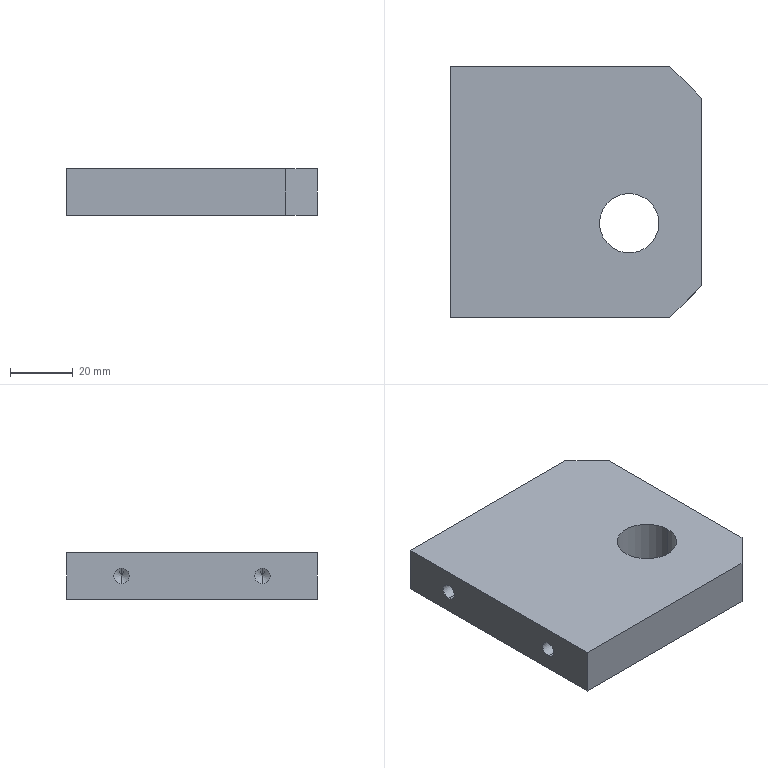Part | STEP file | Lead screw rear fixing plate | 1 solid | 18 faces | box 80 x 80 x 15 mm | volume 89638 mm3 | plane 8 | cylinder 6 | cone 4 | commonest cylinder face diameters 5 x4 19 x2
STEP:
#1=CARTESIAN_POINT('',(0.,0.,0.));
#2=DIRECTION('',(0.,0.,1.));
#3=DIRECTION('',(1.,0.,0.));
#4=AXIS2_PLACEMENT_3D('',#1,#2,#3);
#5=CARTESIAN_POINT('',(-106.907,13.444,5.));
#6=VERTEX_POINT('',#5);
#7=CARTESIAN_POINT('',(-106.907,13.444,10.));
#8=VERTEX_POINT('',#7);
#9=CARTESIAN_POINT('',(-106.907,13.444,7.5));
#10=DIRECTION('',(-1.,0.,0.));
#11=DIRECTION('',(0.,0.,1.));
#12=AXIS2_PLACEMENT_3D('',#9,#10,#11);
#13=CIRCLE('',#12,2.5);
#14=CARTESIAN_POINT('',(-106.907,13.444,7.5));
#15=DIRECTION('',(-1.,0.,0.));
#16=DIRECTION('',(0.,0.,1.));
#17=AXIS2_PLACEMENT_3D('',#14,#15,#16);
#18=CONICAL_SURFACE('',#17,2.5,1.03);
#19=CARTESIAN_POINT('',(0.,0.));
#20=DIRECTION('',(1.,0.));
#21=VECTOR('',#20,1.);
#22=LINE('',#19,#21);
#23=(GEOMETRIC_REPRESENTATION_CONTEXT(2)PARAMETRIC_REPRESENTATION_CONTEXT()REPRESENTATION_CONTEXT('',''));
#24=DEFINITIONAL_REPRESENTATION('',(#22),#23);
#25=PCURVE('',#18,#24);
#26=CARTESIAN_POINT('',(-106.907,13.444,7.5));
#27=DIRECTION('',(-1.,0.,0.));
#28=DIRECTION('',(0.,0.,1.));
#29=AXIS2_PLACEMENT_3D('',#26,#27,#28);
#30=CYLINDRICAL_SURFACE('',#29,2.5);
#31=CARTESIAN_POINT('',(0.,0.));
#32=DIRECTION('',(1.,0.));
#33=VECTOR('',#32,1.);
#34=LINE('',#31,#33);
#35=(GEOMETRIC_REPRESENTATION_CONTEXT(2)PARAMETRIC_REPRESENTATION_CONTEXT()REPRESENTATION_CONTEXT('',''));
#36=DEFINITIONAL_REPRESENTATION('',(#34),#35);
#37=PCURVE('',#30,#36);
#38=SURFACE_CURVE('',#13,(#25,#37),.PCURVE_S1.);
#39=EDGE_CURVE('',#6,#8,#38,.T.);
#40=ORIENTED_EDGE('',*,*,#39,.F.);
#41=CARTESIAN_POINT('',(-105.405,13.444,7.5));
#42=VERTEX_POINT('',#41);
#43=CARTESIAN_POINT('',(-106.907,13.444,5.));
#44=DIRECTION('',(-0.515,0.,-0.8572));
#45=VECTOR('',#44,1.);
#46=LINE('',#43,#45);
#47=CARTESIAN_POINT('',(3.142,0.));
#48=DIRECTION('',(0.,1.));
#49=VECTOR('',#48,1.);
#50=LINE('',#47,#49);
#51=(GEOMETRIC_REPRESENTATION_CONTEXT(2)PARAMETRIC_REPRESENTATION_CONTEXT()REPRESENTATION_CONTEXT('',''));
#52=DEFINITIONAL_REPRESENTATION('',(#50),#51);
#53=PCURVE('',#18,#52);
#54=CARTESIAN_POINT('',(-106.907,13.444,7.5));
#55=DIRECTION('',(-1.,0.,0.));
#56=DIRECTION('',(0.,0.,1.));
#57=AXIS2_PLACEMENT_3D('',#54,#55,#56);
#58=CONICAL_SURFACE('',#57,2.5,1.03);
#59=CARTESIAN_POINT('',(3.142,0.));
#60=DIRECTION('',(0.,1.));
#61=VECTOR('',#60,1.);
#62=LINE('',#59,#61);
#63=(GEOMETRIC_REPRESENTATION_CONTEXT(2)PARAMETRIC_REPRESENTATION_CONTEXT()REPRESENTATION_CONTEXT('',''));
#64=DEFINITIONAL_REPRESENTATION('',(#62),#63);
#65=PCURVE('',#58,#64);
#66=SURFACE_CURVE('',#46,(#53,#65),.PCURVE_S1.);
#67=EDGE_CURVE('',#42,#6,#66,.T.);
#68=ORIENTED_EDGE('',*,*,#67,.F.);
#69=CARTESIAN_POINT('',(-106.907,13.444,10.));
#70=DIRECTION('',(-0.515,0.,0.8572));
#71=VECTOR('',#70,1.);
#72=LINE('',#69,#71);
#73=CARTESIAN_POINT('',(6.283,0.));
#74=DIRECTION('',(0.,1.));
#75=VECTOR('',#74,1.);
#76=LINE('',#73,#75);
#77=(GEOMETRIC_REPRESENTATION_CONTEXT(2)PARAMETRIC_REPRESENTATION_CONTEXT()REPRESENTATION_CONTEXT('',''));
#78=DEFINITIONAL_REPRESENTATION('',(#76),#77);
#79=PCURVE('',#18,#78);
#80=CARTESIAN_POINT('',(0.,0.));
#81=DIRECTION('',(0.,1.));
#82=VECTOR('',#81,1.);
#83=LINE('',#80,#82);
#84=(GEOMETRIC_REPRESENTATION_CONTEXT(2)PARAMETRIC_REPRESENTATION_CONTEXT()REPRESENTATION_CONTEXT('',''));
#85=DEFINITIONAL_REPRESENTATION('',(#83),#84);
#86=PCURVE('',#58,#85);
#87=SURFACE_CURVE('',#72,(#79,#86),.PCURVE_S1.);
#88=EDGE_CURVE('',#42,#8,#87,.T.);
#89=ORIENTED_EDGE('',*,*,#88,.T.);
#90=EDGE_LOOP('',(#40,#68,#89));
#91=FACE_BOUND('',#90,.F.);
#92=ADVANCED_FACE('',(#91),#18,.F.);
#93=CARTESIAN_POINT('',(-106.907,-31.556,5.));
#94=VERTEX_POINT('',#93);
#95=CARTESIAN_POINT('',(-106.907,-31.556,10.));
#96=VERTEX_POINT('',#95);
#97=CARTESIAN_POINT('',(-106.907,-31.556,7.5));
#98=DIRECTION('',(-1.,0.,0.));
#99=DIRECTION('',(0.,0.,1.));
#100=AXIS2_PLACEMENT_3D('',#97,#98,#99);
#101=CIRCLE('',#100,2.5);
#102=CARTESIAN_POINT('',(-106.907,-31.556,7.5));
#103=DIRECTION('',(-1.,0.,0.));
#104=DIRECTION('',(0.,0.,1.));
#105=AXIS2_PLACEMENT_3D('',#102,#103,#104);
#106=CONICAL_SURFACE('',#105,2.5,1.03);
#107=CARTESIAN_POINT('',(0.,0.));
#108=DIRECTION('',(1.,0.));
#109=VECTOR('',#108,1.);
#110=LINE('',#107,#109);
#111=(GEOMETRIC_REPRESENTATION_CONTEXT(2)PARAMETRIC_REPRESENTATION_CONTEXT()REPRESENTATION_CONTEXT('',''));
#112=DEFINITIONAL_REPRESENTATION('',(#110),#111);
#113=PCURVE('',#106,#112);
#114=CARTESIAN_POINT('',(-106.907,-31.556,7.5));
#115=DIRECTION('',(-1.,0.,0.));
#116=DIRECTION('',(0.,0.,1.));
#117=AXIS2_PLACEMENT_3D('',#114,#115,#116);
#118=CYLINDRICAL_SURFACE('',#117,2.5);
#119=CARTESIAN_POINT('',(0.,0.));
#120=DIRECTION('',(1.,0.));
#121=VECTOR('',#120,1.);
#122=LINE('',#119,#121);
#123=(GEOMETRIC_REPRESENTATION_CONTEXT(2)PARAMETRIC_REPRESENTATION_CONTEXT()REPRESENTATION_CONTEXT('',''));
#124=DEFINITIONAL_REPRESENTATION('',(#122),#123);
#125=PCURVE('',#118,#124);
#126=SURFACE_CURVE('',#101,(#113,#125),.PCURVE_S1.);
#127=EDGE_CURVE('',#94,#96,#126,.T.);
#128=ORIENTED_EDGE('',*,*,#127,.F.);
#129=CARTESIAN_POINT('',(-105.405,-31.556,7.5));
#130=VERTEX_POINT('',#129);
#131=CARTESIAN_POINT('',(-106.907,-31.556,5.));
#132=DIRECTION('',(-0.515,0.,-0.8572));
#133=VECTOR('',#132,1.);
#134=LINE('',#131,#133);
#135=CARTESIAN_POINT('',(3.142,0.));
#136=DIRECTION('',(0.,1.));
#137=VECTOR('',#136,1.);
#138=LINE('',#135,#137);
#139=(GEOMETRIC_REPRESENTATION_CONTEXT(2)PARAMETRIC_REPRESENTATION_CONTEXT()REPRESENTATION_CONTEXT('',''));
#140=DEFINITIONAL_REPRESENTATION('',(#138),#139);
#141=PCURVE('',#106,#140);
#142=CARTESIAN_POINT('',(-106.907,-31.556,7.5));
#143=DIRECTION('',(-1.,0.,0.));
#144=DIRECTION('',(0.,0.,1.));
#145=AXIS2_PLACEMENT_3D('',#142,#143,#144);
#146=CONICAL_SURFACE('',#145,2.5,1.03);
#147=CARTESIAN_POINT('',(3.142,0.));
#148=DIRECTION('',(0.,1.));
#149=VECTOR('',#148,1.);
#150=LINE('',#147,#149);
#151=(GEOMETRIC_REPRESENTATION_CONTEXT(2)PARAMETRIC_REPRESENTATION_CONTEXT()REPRESENTATION_CONTEXT('',''));
#152=DEFINITIONAL_REPRESENTATION('',(#150),#151);
#153=PCURVE('',#146,#152);
#154=SURFACE_CURVE('',#134,(#141,#153),.PCURVE_S1.);
#155=EDGE_CURVE('',#130,#94,#154,.T.);
#156=ORIENTED_EDGE('',*,*,#155,.F.);
#157=CARTESIAN_POINT('',(-106.907,-31.556,10.));
#158=DIRECTION('',(-0.515,0.,0.8572));
#159=VECTOR('',#158,1.);
#160=LINE('',#157,#159);
#161=CARTESIAN_POINT('',(6.283,0.));
#162=DIRECTION('',(0.,1.));
#163=VECTOR('',#162,1.);
#164=LINE('',#161,#163);
#165=(GEOMETRIC_REPRESENTATION_CONTEXT(2)PARAMETRIC_REPRESENTATION_CONTEXT()REPRESENTATION_CONTEXT('',''));
#166=DEFINITIONAL_REPRESENTATION('',(#164),#165);
#167=PCURVE('',#106,#166);
#168=CARTESIAN_POINT('',(0.,0.));
#169=DIRECTION('',(0.,1.));
#170=VECTOR('',#169,1.);
#171=LINE('',#168,#170);
#172=(GEOMETRIC_REPRESENTATION_CONTEXT(2)PARAMETRIC_REPRESENTATION_CONTEXT()REPRESENTATION_CONTEXT('',''));
#173=DEFINITIONAL_REPRESENTATION('',(#171),#172);
#174=PCURVE('',#146,#173);
#175=SURFACE_CURVE('',#160,(#167,#174),.PCURVE_S1.);
#176=EDGE_CURVE('',#130,#96,#175,.T.);
#177=ORIENTED_EDGE('',*,*,#176,.T.);
#178=EDGE_LOOP('',(#128,#156,#177));
#179=FACE_BOUND('',#178,.F.);
#180=ADVANCED_FACE('',(#179),#106,.F.);
#181=CARTESIAN_POINT('',(-121.907,-31.556,10.));
#182=VERTEX_POINT('',#181);
#183=CARTESIAN_POINT('',(-106.907,-31.556,10.));
#184=DIRECTION('',(-1.,0.,0.));
#185=VECTOR('',#184,1.);
#186=LINE('',#183,#185);
#187=CARTESIAN_POINT('',(6.283,0.));
#188=DIRECTION('',(0.,1.));
#189=VECTOR('',#188,1.);
#190=LINE('',#187,#189);
#191=(GEOMETRIC_REPRESENTATION_CONTEXT(2)PARAMETRIC_REPRESENTATION_CONTEXT()REPRESENTATION_CONTEXT('',''));
#192=DEFINITIONAL_REPRESENTATION('',(#190),#191);
#193=PCURVE('',#118,#192);
#194=CARTESIAN_POINT('',(-106.907,-31.556,7.5));
#195=DIRECTION('',(-1.,0.,0.));
#196=DIRECTION('',(0.,0.,1.));
#197=AXIS2_PLACEMENT_3D('',#194,#195,#196);
#198=CYLINDRICAL_SURFACE('',#197,2.5);
#199=CARTESIAN_POINT('',(0.,0.));
#200=DIRECTION('',(0.,1.));
#201=VECTOR('',#200,1.);
#202=LINE('',#199,#201);
#203=(GEOMETRIC_REPRESENTATION_CONTEXT(2)PARAMETRIC_REPRESENTATION_CONTEXT()REPRESENTATION_CONTEXT('',''));
#204=DEFINITIONAL_REPRESENTATION('',(#202),#203);
#205=PCURVE('',#198,#204);
#206=SURFACE_CURVE('',#186,(#193,#205),.PCURVE_S1.);
#207=EDGE_CURVE('',#96,#182,#206,.T.);
#208=ORIENTED_EDGE('',*,*,#207,.T.);
#209=CARTESIAN_POINT('',(-121.907,-31.556,5.));
#210=VERTEX_POINT('',#209);
#211=CARTESIAN_POINT('',(-121.907,-31.556,7.5));
#212=DIRECTION('',(-1.,0.,0.));
#213=DIRECTION('',(0.,0.,-1.));
#214=AXIS2_PLACEMENT_3D('',#211,#212,#213);
#215=CIRCLE('',#214,2.5);
#216=CARTESIAN_POINT('',(3.142,15.));
#217=DIRECTION('',(1.,0.));
#218=VECTOR('',#217,1.);
#219=LINE('',#216,#218);
#220=(GEOMETRIC_REPRESENTATION_CONTEXT(2)PARAMETRIC_REPRESENTATION_CONTEXT()REPRESENTATION_CONTEXT('',''));
#221=DEFINITIONAL_REPRESENTATION('',(#219),#220);
#222=PCURVE('',#118,#221);
#223=CARTESIAN_POINT('',(-121.907,-49.056,15.));
#224=DIRECTION('',(1.,0.,0.));
#225=DIRECTION('',(0.,0.,-1.));
#226=AXIS2_PLACEMENT_3D('',#223,#224,#225);
#227=PLANE('',#226);
#228=CARTESIAN_POINT('',(10.,17.5));
#229=CARTESIAN_POINT('',(10.,13.17));
#230=CARTESIAN_POINT('',(6.25,15.335));
#231=CARTESIAN_POINT('',(2.5,17.5));
#232=CARTESIAN_POINT('',(6.25,19.665));
#233=CARTESIAN_POINT('',(10.,21.83));
#234=CARTESIAN_POINT('',(10.,17.5));
#235=(BOUNDED_CURVE()B_SPLINE_CURVE(2,(#228,#229,#230,#231,#232,#233,#234),.UNSPECIFIED.,.T.,.F.)B_SPLINE_CURVE_WITH_KNOTS((1,2,2,2,2,1),(-2.094,0.,2.094,4.189,6.283,8.378),.UNSPECIFIED.)CURVE()GEOMETRIC_REPRESENTATION_ITEM()RATIONAL_B_SPLINE_CURVE((1.,0.5,1.,0.5,1.,0.5,1.))REPRESENTATION_ITEM(''));
#236=(GEOMETRIC_REPRESENTATION_CONTEXT(2)PARAMETRIC_REPRESENTATION_CONTEXT()REPRESENTATION_CONTEXT('',''));
#237=DEFINITIONAL_REPRESENTATION('',(#235),#236);
#238=PCURVE('',#227,#237);
#239=SURFACE_CURVE('',#215,(#222,#238),.PCURVE_S1.);
#240=EDGE_CURVE('',#210,#182,#239,.T.);
#241=ORIENTED_EDGE('',*,*,#240,.F.);
#242=CARTESIAN_POINT('',(-106.907,-31.556,5.));
#243=DIRECTION('',(-1.,0.,0.));
#244=VECTOR('',#243,1.);
#245=LINE('',#242,#244);
#246=CARTESIAN_POINT('',(3.142,0.));
#247=DIRECTION('',(0.,1.));
#248=VECTOR('',#247,1.);
#249=LINE('',#246,#248);
#250=(GEOMETRIC_REPRESENTATION_CONTEXT(2)PARAMETRIC_REPRESENTATION_CONTEXT()REPRESENTATION_CONTEXT('',''));
#251=DEFINITIONAL_REPRESENTATION('',(#249),#250);
#252=PCURVE('',#118,#251);
#253=CARTESIAN_POINT('',(3.142,0.));
#254=DIRECTION('',(0.,1.));
#255=VECTOR('',#254,1.);
#256=LINE('',#253,#255);
#257=(GEOMETRIC_REPRESENTATION_CONTEXT(2)PARAMETRIC_REPRESENTATION_CONTEXT()REPRESENTATION_CONTEXT('',''));
#258=DEFINITIONAL_REPRESENTATION('',(#256),#257);
#259=PCURVE('',#198,#258);
#260=SURFACE_CURVE('',#245,(#252,#259),.PCURVE_S1.);
#261=EDGE_CURVE('',#94,#210,#260,.T.);
#262=ORIENTED_EDGE('',*,*,#261,.F.);
#263=ORIENTED_EDGE('',*,*,#127,.T.);
#264=EDGE_LOOP('',(#208,#241,#262,#263));
#265=FACE_BOUND('',#264,.F.);
#266=ADVANCED_FACE('',(#265),#118,.F.);
#267=CARTESIAN_POINT('',(-121.907,13.444,10.));
#268=VERTEX_POINT('',#267);
#269=CARTESIAN_POINT('',(-106.907,13.444,10.));
#270=DIRECTION('',(-1.,0.,0.));
#271=VECTOR('',#270,1.);
#272=LINE('',#269,#271);
#273=CARTESIAN_POINT('',(6.283,0.));
#274=DIRECTION('',(0.,1.));
#275=VECTOR('',#274,1.);
#276=LINE('',#273,#275);
#277=(GEOMETRIC_REPRESENTATION_CONTEXT(2)PARAMETRIC_REPRESENTATION_CONTEXT()REPRESENTATION_CONTEXT('',''));
#278=DEFINITIONAL_REPRESENTATION('',(#276),#277);
#279=PCURVE('',#30,#278);
#280=CARTESIAN_POINT('',(-106.907,13.444,7.5));
#281=DIRECTION('',(-1.,0.,0.));
#282=DIRECTION('',(0.,0.,1.));
#283=AXIS2_PLACEMENT_3D('',#280,#281,#282);
#284=CYLINDRICAL_SURFACE('',#283,2.5);
#285=CARTESIAN_POINT('',(0.,0.));
#286=DIRECTION('',(0.,1.));
#287=VECTOR('',#286,1.);
#288=LINE('',#285,#287);
#289=(GEOMETRIC_REPRESENTATION_CONTEXT(2)PARAMETRIC_REPRESENTATION_CONTEXT()REPRESENTATION_CONTEXT('',''));
#290=DEFINITIONAL_REPRESENTATION('',(#288),#289);
#291=PCURVE('',#284,#290);
#292=SURFACE_CURVE('',#272,(#279,#291),.PCURVE_S1.);
#293=EDGE_CURVE('',#8,#268,#292,.T.);
#294=ORIENTED_EDGE('',*,*,#293,.T.);
#295=CARTESIAN_POINT('',(-121.907,13.444,5.));
#296=VERTEX_POINT('',#295);
#297=CARTESIAN_POINT('',(-121.907,13.444,7.5));
#298=DIRECTION('',(-1.,0.,0.));
#299=DIRECTION('',(0.,0.,1.));
#300=AXIS2_PLACEMENT_3D('',#297,#298,#299);
#301=CIRCLE('',#300,2.5);
#302=CARTESIAN_POINT('',(0.,15.));
#303=DIRECTION('',(1.,0.));
#304=VECTOR('',#303,1.);
#305=LINE('',#302,#304);
#306=(GEOMETRIC_REPRESENTATION_CONTEXT(2)PARAMETRIC_REPRESENTATION_CONTEXT()REPRESENTATION_CONTEXT('',''));
#307=DEFINITIONAL_REPRESENTATION('',(#305),#306);
#308=PCURVE('',#30,#307);
#309=CARTESIAN_POINT('',(5.,62.5));
#310=CARTESIAN_POINT('',(5.,66.83));
#311=CARTESIAN_POINT('',(8.75,64.665));
#312=CARTESIAN_POINT('',(12.5,62.5));
#313=CARTESIAN_POINT('',(8.75,60.335));
#314=CARTESIAN_POINT('',(5.,58.17));
#315=CARTESIAN_POINT('',(5.,62.5));
#316=(BOUNDED_CURVE()B_SPLINE_CURVE(2,(#309,#310,#311,#312,#313,#314,#315),.UNSPECIFIED.,.T.,.F.)B_SPLINE_CURVE_WITH_KNOTS((1,2,2,2,2,1),(-2.094,0.,2.094,4.189,6.283,8.378),.UNSPECIFIED.)CURVE()GEOMETRIC_REPRESENTATION_ITEM()RATIONAL_B_SPLINE_CURVE((1.,0.5,1.,0.5,1.,0.5,1.))REPRESENTATION_ITEM(''));
#317=(GEOMETRIC_REPRESENTATION_CONTEXT(2)PARAMETRIC_REPRESENTATION_CONTEXT()REPRESENTATION_CONTEXT('',''));
#318=DEFINITIONAL_REPRESENTATION('',(#316),#317);
#319=PCURVE('',#227,#318);
#320=SURFACE_CURVE('',#301,(#308,#319),.PCURVE_S1.);
#321=EDGE_CURVE('',#296,#268,#320,.T.);
#322=ORIENTED_EDGE('',*,*,#321,.F.);
#323=CARTESIAN_POINT('',(-106.907,13.444,5.));
#324=DIRECTION('',(-1.,0.,0.));
#325=VECTOR('',#324,1.);
#326=LINE('',#323,#325);
#327=CARTESIAN_POINT('',(3.142,0.));
#328=DIRECTION('',(0.,1.));
#329=VECTOR('',#328,1.);
#330=LINE('',#327,#329);
#331=(GEOMETRIC_REPRESENTATION_CONTEXT(2)PARAMETRIC_REPRESENTATION_CONTEXT()REPRESENTATION_CONTEXT('',''));
#332=DEFINITIONAL_REPRESENTATION('',(#330),#331);
#333=PCURVE('',#30,#332);
#334=CARTESIAN_POINT('',(3.142,0.));
#335=DIRECTION('',(0.,1.));
#336=VECTOR('',#335,1.);
#337=LINE('',#334,#336);
#338=(GEOMETRIC_REPRESENTATION_CONTEXT(2)PARAMETRIC_REPRESENTATION_CONTEXT()REPRESENTATION_CONTEXT('',''));
#339=DEFINITIONAL_REPRESENTATION('',(#337),#338);
#340=PCURVE('',#284,#339);
#341=SURFACE_CURVE('',#326,(#333,#340),.PCURVE_S1.);
#342=EDGE_CURVE('',#6,#296,#341,.T.);
#343=ORIENTED_EDGE('',*,*,#342,.F.);
#344=ORIENTED_EDGE('',*,*,#39,.T.);
#345=EDGE_LOOP('',(#294,#322,#343,#344));
#346=FACE_BOUND('',#345,.F.);
#347=ADVANCED_FACE('',(#346),#30,.F.);
#348=CARTESIAN_POINT('',(-74.407,-19.056,15.));
#349=VERTEX_POINT('',#348);
#350=CARTESIAN_POINT('',(-74.407,-19.056,0.));
#351=VERTEX_POINT('',#350);
#352=CARTESIAN_POINT('',(-74.407,-19.056,15.));
#353=DIRECTION('',(0.,0.,-1.));
#354=VECTOR('',#353,1.);
#355=LINE('',#352,#354);
#356=CARTESIAN_POINT('',(-64.907,-19.056,15.));
#357=DIRECTION('',(0.,0.,-1.));
#358=DIRECTION('',(-1.,0.,0.));
#359=AXIS2_PLACEMENT_3D('',#356,#357,#358);
#360=CYLINDRICAL_SURFACE('',#359,9.5);
#361=CARTESIAN_POINT('',(6.283,0.));
#362=DIRECTION('',(0.,1.));
#363=VECTOR('',#362,1.);
#364=LINE('',#361,#363);
#365=(GEOMETRIC_REPRESENTATION_CONTEXT(2)PARAMETRIC_REPRESENTATION_CONTEXT()REPRESENTATION_CONTEXT('',''));
#366=DEFINITIONAL_REPRESENTATION('',(#364),#365);
#367=PCURVE('',#360,#366);
#368=CARTESIAN_POINT('',(-64.907,-19.056,15.));
#369=DIRECTION('',(0.,0.,-1.));
#370=DIRECTION('',(-1.,0.,0.));
#371=AXIS2_PLACEMENT_3D('',#368,#369,#370);
#372=CYLINDRICAL_SURFACE('',#371,9.5);
#373=CARTESIAN_POINT('',(0.,0.));
#374=DIRECTION('',(0.,1.));
#375=VECTOR('',#374,1.);
#376=LINE('',#373,#375);
#377=(GEOMETRIC_REPRESENTATION_CONTEXT(2)PARAMETRIC_REPRESENTATION_CONTEXT()REPRESENTATION_CONTEXT('',''));
#378=DEFINITIONAL_REPRESENTATION('',(#376),#377);
#379=PCURVE('',#372,#378);
#380=SURFACE_CURVE('',#355,(#367,#379),.PCURVE_S1.);
#381=EDGE_CURVE('',#349,#351,#380,.T.);
#382=ORIENTED_EDGE('',*,*,#381,.T.);
#383=CARTESIAN_POINT('',(-55.407,-19.056,0.));
#384=VERTEX_POINT('',#383);
#385=CARTESIAN_POINT('',(-64.907,-19.056,0.));
#386=DIRECTION('',(0.,0.,1.));
#387=DIRECTION('',(1.,0.,0.));
#388=AXIS2_PLACEMENT_3D('',#385,#386,#387);
#389=CIRCLE('',#388,9.5);
#390=CARTESIAN_POINT('',(9.425,15.));
#391=DIRECTION('',(-1.,0.));
#392=VECTOR('',#391,1.);
#393=LINE('',#390,#392);
#394=(GEOMETRIC_REPRESENTATION_CONTEXT(2)PARAMETRIC_REPRESENTATION_CONTEXT()REPRESENTATION_CONTEXT('',''));
#395=DEFINITIONAL_REPRESENTATION('',(#393),#394);
#396=PCURVE('',#360,#395);
#397=CARTESIAN_POINT('',(0.,0.,0.));
#398=DIRECTION('',(0.,0.,-1.));
#399=DIRECTION('',(-1.,0.,0.));
#400=AXIS2_PLACEMENT_3D('',#397,#398,#399);
#401=PLANE('',#400);
#402=CARTESIAN_POINT('',(55.407,-19.056));
#403=CARTESIAN_POINT('',(55.407,-2.601));
#404=CARTESIAN_POINT('',(69.657,-10.829));
#405=CARTESIAN_POINT('',(83.907,-19.056));
#406=CARTESIAN_POINT('',(69.657,-27.283));
#407=CARTESIAN_POINT('',(55.407,-35.51));
#408=CARTESIAN_POINT('',(55.407,-19.056));
#409=(BOUNDED_CURVE()B_SPLINE_CURVE(2,(#402,#403,#404,#405,#406,#407,#408),.UNSPECIFIED.,.T.,.F.)B_SPLINE_CURVE_WITH_KNOTS((1,2,2,2,2,1),(-2.094,0.,2.094,4.189,6.283,8.378),.UNSPECIFIED.)CURVE()GEOMETRIC_REPRESENTATION_ITEM()RATIONAL_B_SPLINE_CURVE((1.,0.5,1.,0.5,1.,0.5,1.))REPRESENTATION_ITEM(''));
#410=(GEOMETRIC_REPRESENTATION_CONTEXT(2)PARAMETRIC_REPRESENTATION_CONTEXT()REPRESENTATION_CONTEXT('',''));
#411=DEFINITIONAL_REPRESENTATION('',(#409),#410);
#412=PCURVE('',#401,#411);
#413=SURFACE_CURVE('',#389,(#396,#412),.PCURVE_S1.);
#414=EDGE_CURVE('',#351,#384,#413,.T.);
#415=ORIENTED_EDGE('',*,*,#414,.T.);
#416=CARTESIAN_POINT('',(-55.407,-19.056,15.));
#417=VERTEX_POINT('',#416);
#418=CARTESIAN_POINT('',(-55.407,-19.056,15.));
#419=DIRECTION('',(0.,0.,-1.));
#420=VECTOR('',#419,1.);
#421=LINE('',#418,#420);
#422=CARTESIAN_POINT('',(3.142,0.));
#423=DIRECTION('',(0.,1.));
#424=VECTOR('',#423,1.);
#425=LINE('',#422,#424);
#426=(GEOMETRIC_REPRESENTATION_CONTEXT(2)PARAMETRIC_REPRESENTATION_CONTEXT()REPRESENTATION_CONTEXT('',''));
#427=DEFINITIONAL_REPRESENTATION('',(#425),#426);
#428=PCURVE('',#360,#427);
#429=CARTESIAN_POINT('',(3.142,0.));
#430=DIRECTION('',(0.,1.));
#431=VECTOR('',#430,1.);
#432=LINE('',#429,#431);
#433=(GEOMETRIC_REPRESENTATION_CONTEXT(2)PARAMETRIC_REPRESENTATION_CONTEXT()REPRESENTATION_CONTEXT('',''));
#434=DEFINITIONAL_REPRESENTATION('',(#432),#433);
#435=PCURVE('',#372,#434);
#436=SURFACE_CURVE('',#421,(#428,#435),.PCURVE_S1.);
#437=EDGE_CURVE('',#417,#384,#436,.T.);
#438=ORIENTED_EDGE('',*,*,#437,.F.);
#439=CARTESIAN_POINT('',(-64.907,-19.056,15.));
#440=DIRECTION('',(0.,0.,1.));
#441=DIRECTION('',(1.,0.,0.));
#442=AXIS2_PLACEMENT_3D('',#439,#440,#441);
#443=CIRCLE('',#442,9.5);
#444=CARTESIAN_POINT('',(9.425,0.));
#445=DIRECTION('',(-1.,0.));
#446=VECTOR('',#445,1.);
#447=LINE('',#444,#446);
#448=(GEOMETRIC_REPRESENTATION_CONTEXT(2)PARAMETRIC_REPRESENTATION_CONTEXT()REPRESENTATION_CONTEXT('',''));
#449=DEFINITIONAL_REPRESENTATION('',(#447),#448);
#450=PCURVE('',#360,#449);
#451=CARTESIAN_POINT('',(0.,0.,15.));
#452=DIRECTION('',(0.,0.,-1.));
#453=DIRECTION('',(-1.,0.,0.));
#454=AXIS2_PLACEMENT_3D('',#451,#452,#453);
#455=PLANE('',#454);
#456=CARTESIAN_POINT('',(55.407,-19.056));
#457=CARTESIAN_POINT('',(55.407,-2.601));
#458=CARTESIAN_POINT('',(69.657,-10.829));
#459=CARTESIAN_POINT('',(83.907,-19.056));
#460=CARTESIAN_POINT('',(69.657,-27.283));
#461=CARTESIAN_POINT('',(55.407,-35.51));
#462=CARTESIAN_POINT('',(55.407,-19.056));
#463=(BOUNDED_CURVE()B_SPLINE_CURVE(2,(#456,#457,#458,#459,#460,#461,#462),.UNSPECIFIED.,.T.,.F.)B_SPLINE_CURVE_WITH_KNOTS((1,2,2,2,2,1),(-2.094,0.,2.094,4.189,6.283,8.378),.UNSPECIFIED.)CURVE()GEOMETRIC_REPRESENTATION_ITEM()RATIONAL_B_SPLINE_CURVE((1.,0.5,1.,0.5,1.,0.5,1.))REPRESENTATION_ITEM(''));
#464=(GEOMETRIC_REPRESENTATION_CONTEXT(2)PARAMETRIC_REPRESENTATION_CONTEXT()REPRESENTATION_CONTEXT('',''));
#465=DEFINITIONAL_REPRESENTATION('',(#463),#464);
#466=PCURVE('',#455,#465);
#467=SURFACE_CURVE('',#443,(#450,#466),.PCURVE_S1.);
#468=EDGE_CURVE('',#349,#417,#467,.T.);
#469=ORIENTED_EDGE('',*,*,#468,.F.);
#470=EDGE_LOOP('',(#382,#415,#438,#469));
#471=FACE_BOUND('',#470,.F.);
#472=ADVANCED_FACE('',(#471),#360,.F.);
#473=CARTESIAN_POINT('',(-121.907,30.944,15.));
#474=VERTEX_POINT('',#473);
#475=CARTESIAN_POINT('',(-121.907,-49.056,15.));
#476=VERTEX_POINT('',#475);
#477=CARTESIAN_POINT('',(-121.907,-49.056,15.));
#478=DIRECTION('',(0.,-1.,0.));
#479=VECTOR('',#478,1.);
#480=LINE('',#477,#479);
#481=CARTESIAN_POINT('',(121.907,-49.056));
#482=DIRECTION('',(0.,-1.));
#483=VECTOR('',#482,1.);
#484=LINE('',#481,#483);
#485=(GEOMETRIC_REPRESENTATION_CONTEXT(2)PARAMETRIC_REPRESENTATION_CONTEXT()REPRESENTATION_CONTEXT('',''));
#486=DEFINITIONAL_REPRESENTATION('',(#484),#485);
#487=PCURVE('',#455,#486);
#488=CARTESIAN_POINT('',(0.,0.));
#489=DIRECTION('',(0.,-1.));
#490=VECTOR('',#489,1.);
#491=LINE('',#488,#490);
#492=(GEOMETRIC_REPRESENTATION_CONTEXT(2)PARAMETRIC_REPRESENTATION_CONTEXT()REPRESENTATION_CONTEXT('',''));
#493=DEFINITIONAL_REPRESENTATION('',(#491),#492);
#494=PCURVE('',#227,#493);
#495=SURFACE_CURVE('',#480,(#487,#494),.PCURVE_S1.);
#496=EDGE_CURVE('',#474,#476,#495,.T.);
#497=ORIENTED_EDGE('',*,*,#496,.T.);
#498=CARTESIAN_POINT('',(-51.907,-49.056,15.));
#499=VERTEX_POINT('',#498);
#500=CARTESIAN_POINT('',(-121.907,-49.056,15.));
#501=DIRECTION('',(1.,0.,0.));
#502=VECTOR('',#501,1.);
#503=LINE('',#500,#502);
#504=CARTESIAN_POINT('',(121.907,-49.056));
#505=DIRECTION('',(-1.,0.));
#506=VECTOR('',#505,1.);
#507=LINE('',#504,#506);
#508=(GEOMETRIC_REPRESENTATION_CONTEXT(2)PARAMETRIC_REPRESENTATION_CONTEXT()REPRESENTATION_CONTEXT('',''));
#509=DEFINITIONAL_REPRESENTATION('',(#507),#508);
#510=PCURVE('',#455,#509);
#511=CARTESIAN_POINT('',(-121.907,-49.056,15.));
#512=DIRECTION('',(0.,1.,0.));
#513=DIRECTION('',(0.,0.,1.));
#514=AXIS2_PLACEMENT_3D('',#511,#512,#513);
#515=PLANE('',#514);
#516=CARTESIAN_POINT('',(0.,0.));
#517=DIRECTION('',(0.,1.));
#518=VECTOR('',#517,1.);
#519=LINE('',#516,#518);
#520=(GEOMETRIC_REPRESENTATION_CONTEXT(2)PARAMETRIC_REPRESENTATION_CONTEXT()REPRESENTATION_CONTEXT('',''));
#521=DEFINITIONAL_REPRESENTATION('',(#519),#520);
#522=PCURVE('',#515,#521);
#523=SURFACE_CURVE('',#503,(#510,#522),.PCURVE_S1.);
#524=EDGE_CURVE('',#476,#499,#523,.T.);
#525=ORIENTED_EDGE('',*,*,#524,.T.);
#526=CARTESIAN_POINT('',(-41.907,-39.056,15.));
#527=VERTEX_POINT('',#526);
#528=CARTESIAN_POINT('',(-51.907,-49.056,15.));
#529=DIRECTION('',(0.7071,0.7071,0.));
#530=VECTOR('',#529,1.);
#531=LINE('',#528,#530);
#532=CARTESIAN_POINT('',(51.907,-49.056));
#533=DIRECTION('',(-0.7071,0.7071));
#534=VECTOR('',#533,1.);
#535=LINE('',#532,#534);
#536=(GEOMETRIC_REPRESENTATION_CONTEXT(2)PARAMETRIC_REPRESENTATION_CONTEXT()REPRESENTATION_CONTEXT('',''));
#537=DEFINITIONAL_REPRESENTATION('',(#535),#536);
#538=PCURVE('',#455,#537);
#539=CARTESIAN_POINT('',(-51.907,-49.056,15.));
#540=DIRECTION('',(-0.7071,0.7071,0.));
#541=DIRECTION('',(-0.7071,-0.7071,0.));
#542=AXIS2_PLACEMENT_3D('',#539,#540,#541);
#543=PLANE('',#542);
#544=CARTESIAN_POINT('',(0.,0.));
#545=DIRECTION('',(-1.,0.));
#546=VECTOR('',#545,1.);
#547=LINE('',#544,#546);
#548=(GEOMETRIC_REPRESENTATION_CONTEXT(2)PARAMETRIC_REPRESENTATION_CONTEXT()REPRESENTATION_CONTEXT('',''));
#549=DEFINITIONAL_REPRESENTATION('',(#547),#548);
#550=PCURVE('',#543,#549);
#551=SURFACE_CURVE('',#531,(#538,#550),.PCURVE_S1.);
#552=EDGE_CURVE('',#499,#527,#551,.T.);
#553=ORIENTED_EDGE('',*,*,#552,.T.);
#554=CARTESIAN_POINT('',(-41.907,20.944,15.));
#555=VERTEX_POINT('',#554);
#556=CARTESIAN_POINT('',(-41.907,-39.056,15.));
#557=DIRECTION('',(0.,1.,0.));
#558=VECTOR('',#557,1.);
#559=LINE('',#556,#558);
#560=CARTESIAN_POINT('',(41.907,-39.056));
#561=DIRECTION('',(0.,1.));
#562=VECTOR('',#561,1.);
#563=LINE('',#560,#562);
#564=(GEOMETRIC_REPRESENTATION_CONTEXT(2)PARAMETRIC_REPRESENTATION_CONTEXT()REPRESENTATION_CONTEXT('',''));
#565=DEFINITIONAL_REPRESENTATION('',(#563),#564);
#566=PCURVE('',#455,#565);
#567=CARTESIAN_POINT('',(-41.907,-39.056,15.));
#568=DIRECTION('',(-1.,0.,0.));
#569=DIRECTION('',(0.,0.,1.));
#570=AXIS2_PLACEMENT_3D('',#567,#568,#569);
#571=PLANE('',#570);
#572=CARTESIAN_POINT('',(0.,0.));
#573=DIRECTION('',(0.,1.));
#574=VECTOR('',#573,1.);
#575=LINE('',#572,#574);
#576=(GEOMETRIC_REPRESENTATION_CONTEXT(2)PARAMETRIC_REPRESENTATION_CONTEXT()REPRESENTATION_CONTEXT('',''));
#577=DEFINITIONAL_REPRESENTATION('',(#575),#576);
#578=PCURVE('',#571,#577);
#579=SURFACE_CURVE('',#559,(#566,#578),.PCURVE_S1.);
#580=EDGE_CURVE('',#527,#555,#579,.T.);
#581=ORIENTED_EDGE('',*,*,#580,.T.);
#582=CARTESIAN_POINT('',(-51.907,30.944,15.));
#583=VERTEX_POINT('',#582);
#584=CARTESIAN_POINT('',(-51.907,30.944,15.));
#585=DIRECTION('',(-0.7071,0.7071,0.));
#586=VECTOR('',#585,1.);
#587=LINE('',#584,#586);
#588=CARTESIAN_POINT('',(51.907,30.944));
#589=DIRECTION('',(0.7071,0.7071));
#590=VECTOR('',#589,1.);
#591=LINE('',#588,#590);
#592=(GEOMETRIC_REPRESENTATION_CONTEXT(2)PARAMETRIC_REPRESENTATION_CONTEXT()REPRESENTATION_CONTEXT('',''));
#593=DEFINITIONAL_REPRESENTATION('',(#591),#592);
#594=PCURVE('',#455,#593);
#595=CARTESIAN_POINT('',(-51.907,30.944,15.));
#596=DIRECTION('',(-0.7071,-0.7071,0.));
#597=DIRECTION('',(0.7071,-0.7071,0.));
#598=AXIS2_PLACEMENT_3D('',#595,#596,#597);
#599=PLANE('',#598);
#600=CARTESIAN_POINT('',(0.,0.));
#601=DIRECTION('',(-1.,0.));
#602=VECTOR('',#601,1.);
#603=LINE('',#600,#602);
#604=(GEOMETRIC_REPRESENTATION_CONTEXT(2)PARAMETRIC_REPRESENTATION_CONTEXT()REPRESENTATION_CONTEXT('',''));
#605=DEFINITIONAL_REPRESENTATION('',(#603),#604);
#606=PCURVE('',#599,#605);
#607=SURFACE_CURVE('',#587,(#594,#606),.PCURVE_S1.);
#608=EDGE_CURVE('',#555,#583,#607,.T.);
#609=ORIENTED_EDGE('',*,*,#608,.T.);
#610=CARTESIAN_POINT('',(-121.907,30.944,15.));
#611=DIRECTION('',(-1.,0.,0.));
#612=VECTOR('',#611,1.);
#613=LINE('',#610,#612);
#614=CARTESIAN_POINT('',(121.907,30.944));
#615=DIRECTION('',(1.,0.));
#616=VECTOR('',#615,1.);
#617=LINE('',#614,#616);
#618=(GEOMETRIC_REPRESENTATION_CONTEXT(2)PARAMETRIC_REPRESENTATION_CONTEXT()REPRESENTATION_CONTEXT('',''));
#619=DEFINITIONAL_REPRESENTATION('',(#617),#618);
#620=PCURVE('',#455,#619);
#621=CARTESIAN_POINT('',(-121.907,30.944,15.));
#622=DIRECTION('',(0.,-1.,0.));
#623=DIRECTION('',(0.,0.,-1.));
#624=AXIS2_PLACEMENT_3D('',#621,#622,#623);
#625=PLANE('',#624);
#626=CARTESIAN_POINT('',(0.,0.));
#627=DIRECTION('',(0.,-1.));
#628=VECTOR('',#627,1.);
#629=LINE('',#626,#628);
#630=(GEOMETRIC_REPRESENTATION_CONTEXT(2)PARAMETRIC_REPRESENTATION_CONTEXT()REPRESENTATION_CONTEXT('',''));
#631=DEFINITIONAL_REPRESENTATION('',(#629),#630);
#632=PCURVE('',#625,#631);
#633=SURFACE_CURVE('',#613,(#620,#632),.PCURVE_S1.);
#634=EDGE_CURVE('',#583,#474,#633,.T.);
#635=ORIENTED_EDGE('',*,*,#634,.T.);
#636=EDGE_LOOP('',(#497,#525,#553,#581,#609,#635));
#637=FACE_BOUND('',#636,.T.);
#638=ORIENTED_EDGE('',*,*,#468,.F.);
#639=CARTESIAN_POINT('',(-64.907,-19.056,15.));
#640=DIRECTION('',(0.,0.,1.));
#641=DIRECTION('',(1.,0.,0.));
#642=AXIS2_PLACEMENT_3D('',#639,#640,#641);
#643=CIRCLE('',#642,9.5);
#644=CARTESIAN_POINT('',(55.407,-19.056));
#645=CARTESIAN_POINT('',(55.407,-2.601));
#646=CARTESIAN_POINT('',(69.657,-10.829));
#647=CARTESIAN_POINT('',(83.907,-19.056));
#648=CARTESIAN_POINT('',(69.657,-27.283));
#649=CARTESIAN_POINT('',(55.407,-35.51));
#650=CARTESIAN_POINT('',(55.407,-19.056));
#651=(BOUNDED_CURVE()B_SPLINE_CURVE(2,(#644,#645,#646,#647,#648,#649,#650),.UNSPECIFIED.,.T.,.F.)B_SPLINE_CURVE_WITH_KNOTS((1,2,2,2,2,1),(-2.094,0.,2.094,4.189,6.283,8.378),.UNSPECIFIED.)CURVE()GEOMETRIC_REPRESENTATION_ITEM()RATIONAL_B_SPLINE_CURVE((1.,0.5,1.,0.5,1.,0.5,1.))REPRESENTATION_ITEM(''));
#652=(GEOMETRIC_REPRESENTATION_CONTEXT(2)PARAMETRIC_REPRESENTATION_CONTEXT()REPRESENTATION_CONTEXT('',''));
#653=DEFINITIONAL_REPRESENTATION('',(#651),#652);
#654=PCURVE('',#455,#653);
#655=CARTESIAN_POINT('',(3.142,0.));
#656=DIRECTION('',(-1.,0.));
#657=VECTOR('',#656,1.);
#658=LINE('',#655,#657);
#659=(GEOMETRIC_REPRESENTATION_CONTEXT(2)PARAMETRIC_REPRESENTATION_CONTEXT()REPRESENTATION_CONTEXT('',''));
#660=DEFINITIONAL_REPRESENTATION('',(#658),#659);
#661=PCURVE('',#372,#660);
#662=SURFACE_CURVE('',#643,(#654,#661),.PCURVE_S1.);
#663=EDGE_CURVE('',#417,#349,#662,.T.);
#664=ORIENTED_EDGE('',*,*,#663,.F.);
#665=EDGE_LOOP('',(#638,#664));
#666=FACE_BOUND('',#665,.T.);
#667=ADVANCED_FACE('',(#637,#666),#455,.F.);
#668=CARTESIAN_POINT('',(-121.907,30.944,0.));
#669=VERTEX_POINT('',#668);
#670=CARTESIAN_POINT('',(-121.907,-49.056,0.));
#671=VERTEX_POINT('',#670);
#672=CARTESIAN_POINT('',(-121.907,-49.056,0.));
#673=DIRECTION('',(0.,-1.,0.));
#674=VECTOR('',#673,1.);
#675=LINE('',#672,#674);
#676=CARTESIAN_POINT('',(121.907,-49.056));
#677=DIRECTION('',(0.,-1.));
#678=VECTOR('',#677,1.);
#679=LINE('',#676,#678);
#680=(GEOMETRIC_REPRESENTATION_CONTEXT(2)PARAMETRIC_REPRESENTATION_CONTEXT()REPRESENTATION_CONTEXT('',''));
#681=DEFINITIONAL_REPRESENTATION('',(#679),#680);
#682=PCURVE('',#401,#681);
#683=CARTESIAN_POINT('',(15.,0.));
#684=DIRECTION('',(0.,-1.));
#685=VECTOR('',#684,1.);
#686=LINE('',#683,#685);
#687=(GEOMETRIC_REPRESENTATION_CONTEXT(2)PARAMETRIC_REPRESENTATION_CONTEXT()REPRESENTATION_CONTEXT('',''));
#688=DEFINITIONAL_REPRESENTATION('',(#686),#687);
#689=PCURVE('',#227,#688);
#690=SURFACE_CURVE('',#675,(#682,#689),.PCURVE_S1.);
#691=EDGE_CURVE('',#669,#671,#690,.T.);
#692=ORIENTED_EDGE('',*,*,#691,.F.);
#693=CARTESIAN_POINT('',(-51.907,30.944,0.));
#694=VERTEX_POINT('',#693);
#695=CARTESIAN_POINT('',(-121.907,30.944,0.));
#696=DIRECTION('',(-1.,0.,0.));
#697=VECTOR('',#696,1.);
#698=LINE('',#695,#697);
#699=CARTESIAN_POINT('',(121.907,30.944));
#700=DIRECTION('',(1.,0.));
#701=VECTOR('',#700,1.);
#702=LINE('',#699,#701);
#703=(GEOMETRIC_REPRESENTATION_CONTEXT(2)PARAMETRIC_REPRESENTATION_CONTEXT()REPRESENTATION_CONTEXT('',''));
#704=DEFINITIONAL_REPRESENTATION('',(#702),#703);
#705=PCURVE('',#401,#704);
#706=CARTESIAN_POINT('',(15.,0.));
#707=DIRECTION('',(0.,-1.));
#708=VECTOR('',#707,1.);
#709=LINE('',#706,#708);
#710=(GEOMETRIC_REPRESENTATION_CONTEXT(2)PARAMETRIC_REPRESENTATION_CONTEXT()REPRESENTATION_CONTEXT('',''));
#711=DEFINITIONAL_REPRESENTATION('',(#709),#710);
#712=PCURVE('',#625,#711);
#713=SURFACE_CURVE('',#698,(#705,#712),.PCURVE_S1.);
#714=EDGE_CURVE('',#694,#669,#713,.T.);
#715=ORIENTED_EDGE('',*,*,#714,.F.);
#716=CARTESIAN_POINT('',(-41.907,20.944,0.));
#717=VERTEX_POINT('',#716);
#718=CARTESIAN_POINT('',(-51.907,30.944,0.));
#719=DIRECTION('',(-0.7071,0.7071,0.));
#720=VECTOR('',#719,1.);
#721=LINE('',#718,#720);
#722=CARTESIAN_POINT('',(51.907,30.944));
#723=DIRECTION('',(0.7071,0.7071));
#724=VECTOR('',#723,1.);
#725=LINE('',#722,#724);
#726=(GEOMETRIC_REPRESENTATION_CONTEXT(2)PARAMETRIC_REPRESENTATION_CONTEXT()REPRESENTATION_CONTEXT('',''));
#727=DEFINITIONAL_REPRESENTATION('',(#725),#726);
#728=PCURVE('',#401,#727);
#729=CARTESIAN_POINT('',(0.,-15.));
#730=DIRECTION('',(-1.,0.));
#731=VECTOR('',#730,1.);
#732=LINE('',#729,#731);
#733=(GEOMETRIC_REPRESENTATION_CONTEXT(2)PARAMETRIC_REPRESENTATION_CONTEXT()REPRESENTATION_CONTEXT('',''));
#734=DEFINITIONAL_REPRESENTATION('',(#732),#733);
#735=PCURVE('',#599,#734);
#736=SURFACE_CURVE('',#721,(#728,#735),.PCURVE_S1.);
#737=EDGE_CURVE('',#717,#694,#736,.T.);
#738=ORIENTED_EDGE('',*,*,#737,.F.);
#739=CARTESIAN_POINT('',(-41.907,-39.056,0.));
#740=VERTEX_POINT('',#739);
#741=CARTESIAN_POINT('',(-41.907,-39.056,0.));
#742=DIRECTION('',(0.,1.,0.));
#743=VECTOR('',#742,1.);
#744=LINE('',#741,#743);
#745=CARTESIAN_POINT('',(41.907,-39.056));
#746=DIRECTION('',(0.,1.));
#747=VECTOR('',#746,1.);
#748=LINE('',#745,#747);
#749=(GEOMETRIC_REPRESENTATION_CONTEXT(2)PARAMETRIC_REPRESENTATION_CONTEXT()REPRESENTATION_CONTEXT('',''));
#750=DEFINITIONAL_REPRESENTATION('',(#748),#749);
#751=PCURVE('',#401,#750);
#752=CARTESIAN_POINT('',(-15.,0.));
#753=DIRECTION('',(0.,1.));
#754=VECTOR('',#753,1.);
#755=LINE('',#752,#754);
#756=(GEOMETRIC_REPRESENTATION_CONTEXT(2)PARAMETRIC_REPRESENTATION_CONTEXT()REPRESENTATION_CONTEXT('',''));
#757=DEFINITIONAL_REPRESENTATION('',(#755),#756);
#758=PCURVE('',#571,#757);
#759=SURFACE_CURVE('',#744,(#751,#758),.PCURVE_S1.);
#760=EDGE_CURVE('',#740,#717,#759,.T.);
#761=ORIENTED_EDGE('',*,*,#760,.F.);
#762=CARTESIAN_POINT('',(-51.907,-49.056,0.));
#763=VERTEX_POINT('',#762);
#764=CARTESIAN_POINT('',(-51.907,-49.056,0.));
#765=DIRECTION('',(0.7071,0.7071,0.));
#766=VECTOR('',#765,1.);
#767=LINE('',#764,#766);
#768=CARTESIAN_POINT('',(51.907,-49.056));
#769=DIRECTION('',(-0.7071,0.7071));
#770=VECTOR('',#769,1.);
#771=LINE('',#768,#770);
#772=(GEOMETRIC_REPRESENTATION_CONTEXT(2)PARAMETRIC_REPRESENTATION_CONTEXT()REPRESENTATION_CONTEXT('',''));
#773=DEFINITIONAL_REPRESENTATION('',(#771),#772);
#774=PCURVE('',#401,#773);
#775=CARTESIAN_POINT('',(0.,-15.));
#776=DIRECTION('',(-1.,0.));
#777=VECTOR('',#776,1.);
#778=LINE('',#775,#777);
#779=(GEOMETRIC_REPRESENTATION_CONTEXT(2)PARAMETRIC_REPRESENTATION_CONTEXT()REPRESENTATION_CONTEXT('',''));
#780=DEFINITIONAL_REPRESENTATION('',(#778),#779);
#781=PCURVE('',#543,#780);
#782=SURFACE_CURVE('',#767,(#774,#781),.PCURVE_S1.);
#783=EDGE_CURVE('',#763,#740,#782,.T.);
#784=ORIENTED_EDGE('',*,*,#783,.F.);
#785=CARTESIAN_POINT('',(-121.907,-49.056,0.));
#786=DIRECTION('',(1.,0.,0.));
#787=VECTOR('',#786,1.);
#788=LINE('',#785,#787);
#789=CARTESIAN_POINT('',(121.907,-49.056));
#790=DIRECTION('',(-1.,0.));
#791=VECTOR('',#790,1.);
#792=LINE('',#789,#791);
#793=(GEOMETRIC_REPRESENTATION_CONTEXT(2)PARAMETRIC_REPRESENTATION_CONTEXT()REPRESENTATION_CONTEXT('',''));
#794=DEFINITIONAL_REPRESENTATION('',(#792),#793);
#795=PCURVE('',#401,#794);
#796=CARTESIAN_POINT('',(-15.,0.));
#797=DIRECTION('',(0.,1.));
#798=VECTOR('',#797,1.);
#799=LINE('',#796,#798);
#800=(GEOMETRIC_REPRESENTATION_CONTEXT(2)PARAMETRIC_REPRESENTATION_CONTEXT()REPRESENTATION_CONTEXT('',''));
#801=DEFINITIONAL_REPRESENTATION('',(#799),#800);
#802=PCURVE('',#515,#801);
#803=SURFACE_CURVE('',#788,(#795,#802),.PCURVE_S1.);
#804=EDGE_CURVE('',#671,#763,#803,.T.);
#805=ORIENTED_EDGE('',*,*,#804,.F.);
#806=EDGE_LOOP('',(#692,#715,#738,#761,#784,#805));
#807=FACE_BOUND('',#806,.T.);
#808=ORIENTED_EDGE('',*,*,#414,.T.);
#809=CARTESIAN_POINT('',(-64.907,-19.056,0.));
#810=DIRECTION('',(0.,0.,1.));
#811=DIRECTION('',(1.,0.,0.));
#812=AXIS2_PLACEMENT_3D('',#809,#810,#811);
#813=CIRCLE('',#812,9.5);
#814=CARTESIAN_POINT('',(55.407,-19.056));
#815=CARTESIAN_POINT('',(55.407,-2.601));
#816=CARTESIAN_POINT('',(69.657,-10.829));
#817=CARTESIAN_POINT('',(83.907,-19.056));
#818=CARTESIAN_POINT('',(69.657,-27.283));
#819=CARTESIAN_POINT('',(55.407,-35.51));
#820=CARTESIAN_POINT('',(55.407,-19.056));
#821=(BOUNDED_CURVE()B_SPLINE_CURVE(2,(#814,#815,#816,#817,#818,#819,#820),.UNSPECIFIED.,.T.,.F.)B_SPLINE_CURVE_WITH_KNOTS((1,2,2,2,2,1),(-2.094,0.,2.094,4.189,6.283,8.378),.UNSPECIFIED.)CURVE()GEOMETRIC_REPRESENTATION_ITEM()RATIONAL_B_SPLINE_CURVE((1.,0.5,1.,0.5,1.,0.5,1.))REPRESENTATION_ITEM(''));
#822=(GEOMETRIC_REPRESENTATION_CONTEXT(2)PARAMETRIC_REPRESENTATION_CONTEXT()REPRESENTATION_CONTEXT('',''));
#823=DEFINITIONAL_REPRESENTATION('',(#821),#822);
#824=PCURVE('',#401,#823);
#825=CARTESIAN_POINT('',(3.142,15.));
#826=DIRECTION('',(-1.,0.));
#827=VECTOR('',#826,1.);
#828=LINE('',#825,#827);
#829=(GEOMETRIC_REPRESENTATION_CONTEXT(2)PARAMETRIC_REPRESENTATION_CONTEXT()REPRESENTATION_CONTEXT('',''));
#830=DEFINITIONAL_REPRESENTATION('',(#828),#829);
#831=PCURVE('',#372,#830);
#832=SURFACE_CURVE('',#813,(#824,#831),.PCURVE_S1.);
#833=EDGE_CURVE('',#384,#351,#832,.T.);
#834=ORIENTED_EDGE('',*,*,#833,.T.);
#835=EDGE_LOOP('',(#808,#834));
#836=FACE_BOUND('',#835,.T.);
#837=ADVANCED_FACE('',(#807,#836),#401,.T.);
#838=CARTESIAN_POINT('',(-121.907,-31.556,7.5));
#839=DIRECTION('',(-1.,0.,0.));
#840=DIRECTION('',(0.,0.,-1.));
#841=AXIS2_PLACEMENT_3D('',#838,#839,#840);
#842=CIRCLE('',#841,2.5);
#843=CARTESIAN_POINT('',(10.,17.5));
#844=CARTESIAN_POINT('',(10.,13.17));
#845=CARTESIAN_POINT('',(6.25,15.335));
#846=CARTESIAN_POINT('',(2.5,17.5));
#847=CARTESIAN_POINT('',(6.25,19.665));
#848=CARTESIAN_POINT('',(10.,21.83));
#849=CARTESIAN_POINT('',(10.,17.5));
#850=(BOUNDED_CURVE()B_SPLINE_CURVE(2,(#843,#844,#845,#846,#847,#848,#849),.UNSPECIFIED.,.T.,.F.)B_SPLINE_CURVE_WITH_KNOTS((1,2,2,2,2,1),(-2.094,0.,2.094,4.189,6.283,8.378),.UNSPECIFIED.)CURVE()GEOMETRIC_REPRESENTATION_ITEM()RATIONAL_B_SPLINE_CURVE((1.,0.5,1.,0.5,1.,0.5,1.))REPRESENTATION_ITEM(''));
#851=(GEOMETRIC_REPRESENTATION_CONTEXT(2)PARAMETRIC_REPRESENTATION_CONTEXT()REPRESENTATION_CONTEXT('',''));
#852=DEFINITIONAL_REPRESENTATION('',(#850),#851);
#853=PCURVE('',#227,#852);
#854=CARTESIAN_POINT('',(-3.142,15.));
#855=DIRECTION('',(1.,0.));
#856=VECTOR('',#855,1.);
#857=LINE('',#854,#856);
#858=(GEOMETRIC_REPRESENTATION_CONTEXT(2)PARAMETRIC_REPRESENTATION_CONTEXT()REPRESENTATION_CONTEXT('',''));
#859=DEFINITIONAL_REPRESENTATION('',(#857),#858);
#860=PCURVE('',#198,#859);
#861=SURFACE_CURVE('',#842,(#853,#860),.PCURVE_S1.);
#862=EDGE_CURVE('',#182,#210,#861,.T.);
#863=ORIENTED_EDGE('',*,*,#862,.F.);
#864=ORIENTED_EDGE('',*,*,#240,.F.);
#865=EDGE_LOOP('',(#863,#864));
#866=FACE_BOUND('',#865,.T.);
#867=CARTESIAN_POINT('',(-121.907,13.444,7.5));
#868=DIRECTION('',(-1.,0.,0.));
#869=DIRECTION('',(0.,0.,1.));
#870=AXIS2_PLACEMENT_3D('',#867,#868,#869);
#871=CIRCLE('',#870,2.5);
#872=CARTESIAN_POINT('',(5.,62.5));
#873=CARTESIAN_POINT('',(5.,66.83));
#874=CARTESIAN_POINT('',(8.75,64.665));
#875=CARTESIAN_POINT('',(12.5,62.5));
#876=CARTESIAN_POINT('',(8.75,60.335));
#877=CARTESIAN_POINT('',(5.,58.17));
#878=CARTESIAN_POINT('',(5.,62.5));
#879=(BOUNDED_CURVE()B_SPLINE_CURVE(2,(#872,#873,#874,#875,#876,#877,#878),.UNSPECIFIED.,.T.,.F.)B_SPLINE_CURVE_WITH_KNOTS((1,2,2,2,2,1),(-2.094,0.,2.094,4.189,6.283,8.378),.UNSPECIFIED.)CURVE()GEOMETRIC_REPRESENTATION_ITEM()RATIONAL_B_SPLINE_CURVE((1.,0.5,1.,0.5,1.,0.5,1.))REPRESENTATION_ITEM(''));
#880=(GEOMETRIC_REPRESENTATION_CONTEXT(2)PARAMETRIC_REPRESENTATION_CONTEXT()REPRESENTATION_CONTEXT('',''));
#881=DEFINITIONAL_REPRESENTATION('',(#879),#880);
#882=PCURVE('',#227,#881);
#883=CARTESIAN_POINT('',(0.,15.));
#884=DIRECTION('',(1.,0.));
#885=VECTOR('',#884,1.);
#886=LINE('',#883,#885);
#887=(GEOMETRIC_REPRESENTATION_CONTEXT(2)PARAMETRIC_REPRESENTATION_CONTEXT()REPRESENTATION_CONTEXT('',''));
#888=DEFINITIONAL_REPRESENTATION('',(#886),#887);
#889=PCURVE('',#284,#888);
#890=SURFACE_CURVE('',#871,(#882,#889),.PCURVE_S1.);
#891=EDGE_CURVE('',#268,#296,#890,.T.);
#892=ORIENTED_EDGE('',*,*,#891,.F.);
#893=ORIENTED_EDGE('',*,*,#321,.F.);
#894=EDGE_LOOP('',(#892,#893));
#895=FACE_BOUND('',#894,.T.);
#896=ORIENTED_EDGE('',*,*,#691,.T.);
#897=CARTESIAN_POINT('',(-121.907,-49.056,15.));
#898=DIRECTION('',(0.,0.,-1.));
#899=VECTOR('',#898,1.);
#900=LINE('',#897,#899);
#901=CARTESIAN_POINT('',(0.,0.));
#902=DIRECTION('',(1.,0.));
#903=VECTOR('',#902,1.);
#904=LINE('',#901,#903);
#905=(GEOMETRIC_REPRESENTATION_CONTEXT(2)PARAMETRIC_REPRESENTATION_CONTEXT()REPRESENTATION_CONTEXT('',''));
#906=DEFINITIONAL_REPRESENTATION('',(#904),#905);
#907=PCURVE('',#227,#906);
#908=CARTESIAN_POINT('',(0.,0.));
#909=DIRECTION('',(-1.,0.));
#910=VECTOR('',#909,1.);
#911=LINE('',#908,#910);
#912=(GEOMETRIC_REPRESENTATION_CONTEXT(2)PARAMETRIC_REPRESENTATION_CONTEXT()REPRESENTATION_CONTEXT('',''));
#913=DEFINITIONAL_REPRESENTATION('',(#911),#912);
#914=PCURVE('',#515,#913);
#915=SURFACE_CURVE('',#900,(#907,#914),.PCURVE_S1.);
#916=EDGE_CURVE('',#476,#671,#915,.T.);
#917=ORIENTED_EDGE('',*,*,#916,.F.);
#918=ORIENTED_EDGE('',*,*,#496,.F.);
#919=CARTESIAN_POINT('',(-121.907,30.944,15.));
#920=DIRECTION('',(0.,0.,-1.));
#921=VECTOR('',#920,1.);
#922=LINE('',#919,#921);
#923=CARTESIAN_POINT('',(0.,80.));
#924=DIRECTION('',(1.,0.));
#925=VECTOR('',#924,1.);
#926=LINE('',#923,#925);
#927=(GEOMETRIC_REPRESENTATION_CONTEXT(2)PARAMETRIC_REPRESENTATION_CONTEXT()REPRESENTATION_CONTEXT('',''));
#928=DEFINITIONAL_REPRESENTATION('',(#926),#927);
#929=PCURVE('',#227,#928);
#930=CARTESIAN_POINT('',(0.,0.));
#931=DIRECTION('',(1.,0.));
#932=VECTOR('',#931,1.);
#933=LINE('',#930,#932);
#934=(GEOMETRIC_REPRESENTATION_CONTEXT(2)PARAMETRIC_REPRESENTATION_CONTEXT()REPRESENTATION_CONTEXT('',''));
#935=DEFINITIONAL_REPRESENTATION('',(#933),#934);
#936=PCURVE('',#625,#935);
#937=SURFACE_CURVE('',#922,(#929,#936),.PCURVE_S1.);
#938=EDGE_CURVE('',#474,#669,#937,.T.);
#939=ORIENTED_EDGE('',*,*,#938,.T.);
#940=EDGE_LOOP('',(#896,#917,#918,#939));
#941=FACE_BOUND('',#940,.T.);
#942=ADVANCED_FACE('',(#866,#895,#941),#227,.F.);
#943=ORIENTED_EDGE('',*,*,#804,.T.);
#944=CARTESIAN_POINT('',(-51.907,-49.056,15.));
#945=DIRECTION('',(0.,0.,-1.));
#946=VECTOR('',#945,1.);
#947=LINE('',#944,#946);
#948=CARTESIAN_POINT('',(0.,70.));
#949=DIRECTION('',(-1.,0.));
#950=VECTOR('',#949,1.);
#951=LINE('',#948,#950);
#952=(GEOMETRIC_REPRESENTATION_CONTEXT(2)PARAMETRIC_REPRESENTATION_CONTEXT()REPRESENTATION_CONTEXT('',''));
#953=DEFINITIONAL_REPRESENTATION('',(#951),#952);
#954=PCURVE('',#515,#953);
#955=CARTESIAN_POINT('',(0.,0.));
#956=DIRECTION('',(0.,-1.));
#957=VECTOR('',#956,1.);
#958=LINE('',#955,#957);
#959=(GEOMETRIC_REPRESENTATION_CONTEXT(2)PARAMETRIC_REPRESENTATION_CONTEXT()REPRESENTATION_CONTEXT('',''));
#960=DEFINITIONAL_REPRESENTATION('',(#958),#959);
#961=PCURVE('',#543,#960);
#962=SURFACE_CURVE('',#947,(#954,#961),.PCURVE_S1.);
#963=EDGE_CURVE('',#499,#763,#962,.T.);
#964=ORIENTED_EDGE('',*,*,#963,.F.);
#965=ORIENTED_EDGE('',*,*,#524,.F.);
#966=ORIENTED_EDGE('',*,*,#916,.T.);
#967=EDGE_LOOP('',(#943,#964,#965,#966));
#968=FACE_BOUND('',#967,.T.);
#969=ADVANCED_FACE('',(#968),#515,.F.);
#970=ORIENTED_EDGE('',*,*,#783,.T.);
#971=CARTESIAN_POINT('',(-41.907,-39.056,15.));
#972=DIRECTION('',(0.,0.,-1.));
#973=VECTOR('',#972,1.);
#974=LINE('',#971,#973);
#975=CARTESIAN_POINT('',(-14.142,0.));
#976=DIRECTION('',(0.,-1.));
#977=VECTOR('',#976,1.);
#978=LINE('',#975,#977);
#979=(GEOMETRIC_REPRESENTATION_CONTEXT(2)PARAMETRIC_REPRESENTATION_CONTEXT()REPRESENTATION_CONTEXT('',''));
#980=DEFINITIONAL_REPRESENTATION('',(#978),#979);
#981=PCURVE('',#543,#980);
#982=CARTESIAN_POINT('',(0.,0.));
#983=DIRECTION('',(-1.,0.));
#984=VECTOR('',#983,1.);
#985=LINE('',#982,#984);
#986=(GEOMETRIC_REPRESENTATION_CONTEXT(2)PARAMETRIC_REPRESENTATION_CONTEXT()REPRESENTATION_CONTEXT('',''));
#987=DEFINITIONAL_REPRESENTATION('',(#985),#986);
#988=PCURVE('',#571,#987);
#989=SURFACE_CURVE('',#974,(#981,#988),.PCURVE_S1.);
#990=EDGE_CURVE('',#527,#740,#989,.T.);
#991=ORIENTED_EDGE('',*,*,#990,.F.);
#992=ORIENTED_EDGE('',*,*,#552,.F.);
#993=ORIENTED_EDGE('',*,*,#963,.T.);
#994=EDGE_LOOP('',(#970,#991,#992,#993));
#995=FACE_BOUND('',#994,.T.);
#996=ADVANCED_FACE('',(#995),#543,.F.);
#997=ORIENTED_EDGE('',*,*,#760,.T.);
#998=CARTESIAN_POINT('',(-41.907,20.944,15.));
#999=DIRECTION('',(0.,0.,-1.));
#1000=VECTOR('',#999,1.);
#1001=LINE('',#998,#1000);
#1002=CARTESIAN_POINT('',(0.,60.));
#1003=DIRECTION('',(-1.,0.));
#1004=VECTOR('',#1003,1.);
#1005=LINE('',#1002,#1004);
#1006=(GEOMETRIC_REPRESENTATION_CONTEXT(2)PARAMETRIC_REPRESENTATION_CONTEXT()REPRESENTATION_CONTEXT('',''));
#1007=DEFINITIONAL_REPRESENTATION('',(#1005),#1006);
#1008=PCURVE('',#571,#1007);
#1009=CARTESIAN_POINT('',(14.142,0.));
#1010=DIRECTION('',(0.,-1.));
#1011=VECTOR('',#1010,1.);
#1012=LINE('',#1009,#1011);
#1013=(GEOMETRIC_REPRESENTATION_CONTEXT(2)PARAMETRIC_REPRESENTATION_CONTEXT()REPRESENTATION_CONTEXT('',''));
#1014=DEFINITIONAL_REPRESENTATION('',(#1012),#1013);
#1015=PCURVE('',#599,#1014);
#1016=SURFACE_CURVE('',#1001,(#1008,#1015),.PCURVE_S1.);
#1017=EDGE_CURVE('',#555,#717,#1016,.T.);
#1018=ORIENTED_EDGE('',*,*,#1017,.F.);
#1019=ORIENTED_EDGE('',*,*,#580,.F.);
#1020=ORIENTED_EDGE('',*,*,#990,.T.);
#1021=EDGE_LOOP('',(#997,#1018,#1019,#1020));
#1022=FACE_BOUND('',#1021,.T.);
#1023=ADVANCED_FACE('',(#1022),#571,.F.);
#1024=ORIENTED_EDGE('',*,*,#737,.T.);
#1025=CARTESIAN_POINT('',(-51.907,30.944,15.));
#1026=DIRECTION('',(0.,0.,-1.));
#1027=VECTOR('',#1026,1.);
#1028=LINE('',#1025,#1027);
#1029=CARTESIAN_POINT('',(0.,0.));
#1030=DIRECTION('',(0.,-1.));
#1031=VECTOR('',#1030,1.);
#1032=LINE('',#1029,#1031);
#1033=(GEOMETRIC_REPRESENTATION_CONTEXT(2)PARAMETRIC_REPRESENTATION_CONTEXT()REPRESENTATION_CONTEXT('',''));
#1034=DEFINITIONAL_REPRESENTATION('',(#1032),#1033);
#1035=PCURVE('',#599,#1034);
#1036=CARTESIAN_POINT('',(0.,70.));
#1037=DIRECTION('',(1.,0.));
#1038=VECTOR('',#1037,1.);
#1039=LINE('',#1036,#1038);
#1040=(GEOMETRIC_REPRESENTATION_CONTEXT(2)PARAMETRIC_REPRESENTATION_CONTEXT()REPRESENTATION_CONTEXT('',''));
#1041=DEFINITIONAL_REPRESENTATION('',(#1039),#1040);
#1042=PCURVE('',#625,#1041);
#1043=SURFACE_CURVE('',#1028,(#1035,#1042),.PCURVE_S1.);
#1044=EDGE_CURVE('',#583,#694,#1043,.T.);
#1045=ORIENTED_EDGE('',*,*,#1044,.F.);
#1046=ORIENTED_EDGE('',*,*,#608,.F.);
#1047=ORIENTED_EDGE('',*,*,#1017,.T.);
#1048=EDGE_LOOP('',(#1024,#1045,#1046,#1047));
#1049=FACE_BOUND('',#1048,.T.);
#1050=ADVANCED_FACE('',(#1049),#599,.F.);
#1051=ORIENTED_EDGE('',*,*,#714,.T.);
#1052=ORIENTED_EDGE('',*,*,#938,.F.);
#1053=ORIENTED_EDGE('',*,*,#634,.F.);
#1054=ORIENTED_EDGE('',*,*,#1044,.T.);
#1055=EDGE_LOOP('',(#1051,#1052,#1053,#1054));
#1056=FACE_BOUND('',#1055,.T.);
#1057=ADVANCED_FACE('',(#1056),#625,.F.);
#1058=ORIENTED_EDGE('',*,*,#833,.T.);
#1059=ORIENTED_EDGE('',*,*,#381,.F.);
#1060=ORIENTED_EDGE('',*,*,#663,.F.);
#1061=ORIENTED_EDGE('',*,*,#437,.T.);
#1062=EDGE_LOOP('',(#1058,#1059,#1060,#1061));
#1063=FACE_BOUND('',#1062,.F.);
#1064=ADVANCED_FACE('',(#1063),#372,.F.);
#1065=ORIENTED_EDGE('',*,*,#891,.F.);
#1066=ORIENTED_EDGE('',*,*,#293,.F.);
#1067=CARTESIAN_POINT('',(-106.907,13.444,7.5));
#1068=DIRECTION('',(-1.,0.,0.));
#1069=DIRECTION('',(0.,0.,1.));
#1070=AXIS2_PLACEMENT_3D('',#1067,#1068,#1069);
#1071=CIRCLE('',#1070,2.5);
#1072=CARTESIAN_POINT('',(0.,0.));
#1073=DIRECTION('',(1.,0.));
#1074=VECTOR('',#1073,1.);
#1075=LINE('',#1072,#1074);
#1076=(GEOMETRIC_REPRESENTATION_CONTEXT(2)PARAMETRIC_REPRESENTATION_CONTEXT()REPRESENTATION_CONTEXT('',''));
#1077=DEFINITIONAL_REPRESENTATION('',(#1075),#1076);
#1078=PCURVE('',#284,#1077);
#1079=CARTESIAN_POINT('',(0.,0.));
#1080=DIRECTION('',(1.,0.));
#1081=VECTOR('',#1080,1.);
#1082=LINE('',#1079,#1081);
#1083=(GEOMETRIC_REPRESENTATION_CONTEXT(2)PARAMETRIC_REPRESENTATION_CONTEXT()REPRESENTATION_CONTEXT('',''));
#1084=DEFINITIONAL_REPRESENTATION('',(#1082),#1083);
#1085=PCURVE('',#58,#1084);
#1086=SURFACE_CURVE('',#1071,(#1078,#1085),.PCURVE_S1.);
#1087=EDGE_CURVE('',#8,#6,#1086,.T.);
#1088=ORIENTED_EDGE('',*,*,#1087,.T.);
#1089=ORIENTED_EDGE('',*,*,#342,.T.);
#1090=EDGE_LOOP('',(#1065,#1066,#1088,#1089));
#1091=FACE_BOUND('',#1090,.F.);
#1092=ADVANCED_FACE('',(#1091),#284,.F.);
#1093=ORIENTED_EDGE('',*,*,#862,.F.);
#1094=ORIENTED_EDGE('',*,*,#207,.F.);
#1095=CARTESIAN_POINT('',(-106.907,-31.556,7.5));
#1096=DIRECTION('',(-1.,0.,0.));
#1097=DIRECTION('',(0.,0.,1.));
#1098=AXIS2_PLACEMENT_3D('',#1095,#1096,#1097);
#1099=CIRCLE('',#1098,2.5);
#1100=CARTESIAN_POINT('',(0.,0.));
#1101=DIRECTION('',(1.,0.));
#1102=VECTOR('',#1101,1.);
#1103=LINE('',#1100,#1102);
#1104=(GEOMETRIC_REPRESENTATION_CONTEXT(2)PARAMETRIC_REPRESENTATION_CONTEXT()REPRESENTATION_CONTEXT('',''));
#1105=DEFINITIONAL_REPRESENTATION('',(#1103),#1104);
#1106=PCURVE('',#198,#1105);
#1107=CARTESIAN_POINT('',(0.,0.));
#1108=DIRECTION('',(1.,0.));
#1109=VECTOR('',#1108,1.);
#1110=LINE('',#1107,#1109);
#1111=(GEOMETRIC_REPRESENTATION_CONTEXT(2)PARAMETRIC_REPRESENTATION_CONTEXT()REPRESENTATION_CONTEXT('',''));
#1112=DEFINITIONAL_REPRESENTATION('',(#1110),#1111);
#1113=PCURVE('',#146,#1112);
#1114=SURFACE_CURVE('',#1099,(#1106,#1113),.PCURVE_S1.);
#1115=EDGE_CURVE('',#96,#94,#1114,.T.);
#1116=ORIENTED_EDGE('',*,*,#1115,.T.);
#1117=ORIENTED_EDGE('',*,*,#261,.T.);
#1118=EDGE_LOOP('',(#1093,#1094,#1116,#1117));
#1119=FACE_BOUND('',#1118,.F.);
#1120=ADVANCED_FACE('',(#1119),#198,.F.);
#1121=ORIENTED_EDGE('',*,*,#1115,.F.);
#1122=ORIENTED_EDGE('',*,*,#176,.F.);
#1123=ORIENTED_EDGE('',*,*,#155,.T.);
#1124=EDGE_LOOP('',(#1121,#1122,#1123));
#1125=FACE_BOUND('',#1124,.F.);
#1126=ADVANCED_FACE('',(#1125),#146,.F.);
#1127=ORIENTED_EDGE('',*,*,#1087,.F.);
#1128=ORIENTED_EDGE('',*,*,#88,.F.);
#1129=ORIENTED_EDGE('',*,*,#67,.T.);
#1130=EDGE_LOOP('',(#1127,#1128,#1129));
#1131=FACE_BOUND('',#1130,.F.);
#1132=ADVANCED_FACE('',(#1131),#58,.F.);
#1133=CLOSED_SHELL('',(#92,#180,#266,#347,#472,#667,#837,#942,#969,#996,#1023,#1050,#1057,#1064,#1092,#1120,#1126,#1132));
#1134=MANIFOLD_SOLID_BREP('',#1133);
#1135=(LENGTH_UNIT()NAMED_UNIT(*)SI_UNIT(.MILLI.,.METRE.));
#1136=UNCERTAINTY_MEASURE_WITH_UNIT(LENGTH_MEASURE(0.0000001),#1135,'','');
#1137=(NAMED_UNIT(*)PLANE_ANGLE_UNIT()SI_UNIT($,.RADIAN.));
#1138=(NAMED_UNIT(*)SI_UNIT($,.STERADIAN.)SOLID_ANGLE_UNIT());
#1139=(GEOMETRIC_REPRESENTATION_CONTEXT(3)GLOBAL_UNCERTAINTY_ASSIGNED_CONTEXT((#1136))GLOBAL_UNIT_ASSIGNED_CONTEXT((#1135,#1137,#1138))REPRESENTATION_CONTEXT('',''));
#1140=ADVANCED_BREP_SHAPE_REPRESENTATION('',(#4,#1134),#1139);